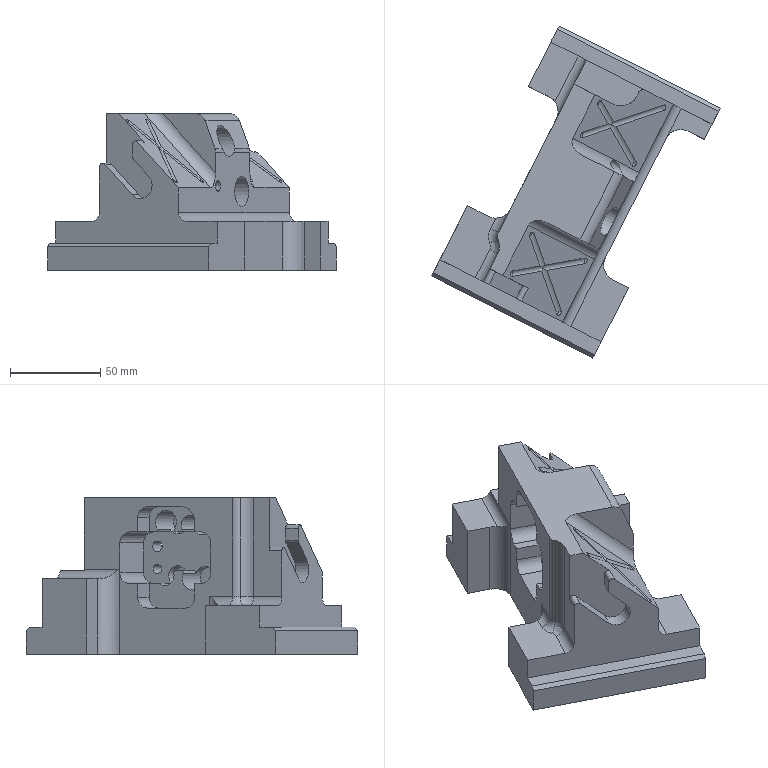Part | STEP file | gslz 2016.10.28-13_id1766_x_t | 1 solid | 149 faces | box 159.469 x 183.505 x 86.5 mm | volume 557397 mm3 | plane 70 | cylinder 65 | sphere 8 | cone 4 | torus 1 | spline 1 | commonest cylinder face diameters 6 x19 12 x12 2 x6 4 x5 10 x5 18 x5